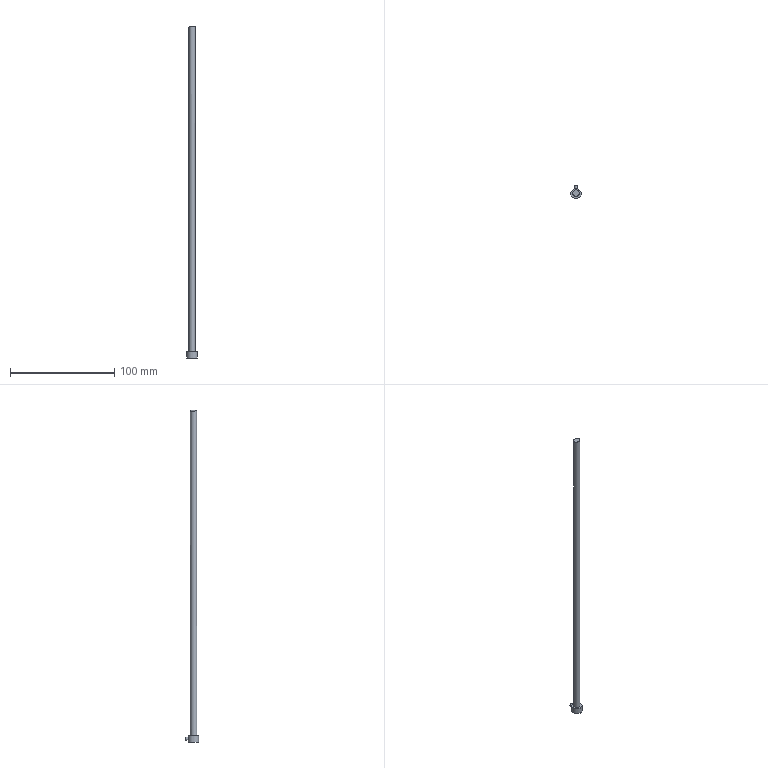Part | STEP file | E106-26-325 | 1 solid | 8 faces | box 10 x 13 x 318.085 mm | volume 9301 mm3 | cylinder 3 | plane 3 | spline 1 | cone 1 | commonest cylinder face diameters 3 x1 6 x1 10 x1